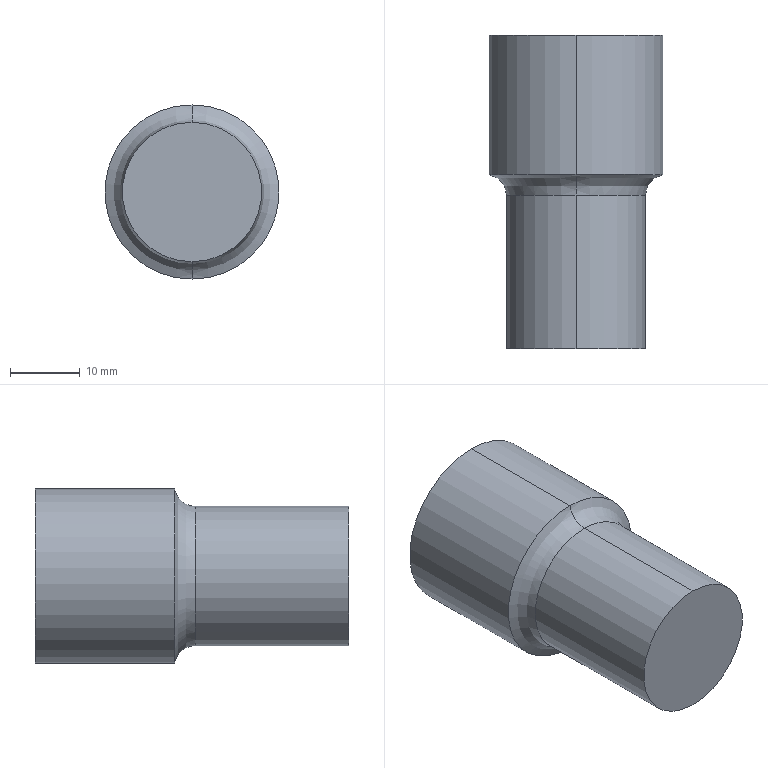Part | SolidWorks | features Fillet 1, Revolution 1 | 1 solid | 8 faces | box 25 x 45 x 25 mm | volume 17793 mm3 | cylinder 4 | torus 2 | plane 2 | commonest cylinder face diameters 20 x2 25 x2
STEP:
#1=CARTESIAN_POINT('',(0.,-6.354,-12.5));
#2=VERTEX_POINT('',#1);
#3=CARTESIAN_POINT('',(0.,-6.354,12.5));
#4=VERTEX_POINT('',#3);
#5=CARTESIAN_POINT('',(0.,-6.354,0.));
#6=DIRECTION('',(0.,1.,0.));
#7=DIRECTION('',(0.,0.,1.));
#8=AXIS2_PLACEMENT_3D('',#5,#6,#7);
#9=CIRCLE('',#8,12.5);
#10=EDGE_CURVE('',#2,#4,#9,.T.);
#11=ORIENTED_EDGE('',*,*,#10,.F.);
#12=CARTESIAN_POINT('',(0.,-9.312,-10.));
#13=VERTEX_POINT('',#12);
#14=CARTESIAN_POINT('',(0.,-9.312,-13.));
#15=DIRECTION('',(1.,0.,0.));
#16=DIRECTION('',(0.,0.,-1.));
#17=AXIS2_PLACEMENT_3D('',#14,#15,#16);
#18=CIRCLE('',#17,3.);
#19=EDGE_CURVE('',#2,#13,#18,.T.);
#20=ORIENTED_EDGE('',*,*,#19,.T.);
#21=CARTESIAN_POINT('',(0.,-9.312,10.));
#22=VERTEX_POINT('',#21);
#23=CARTESIAN_POINT('',(0.,-9.312,0.));
#24=DIRECTION('',(0.,-1.,0.));
#25=DIRECTION('',(0.,0.,1.));
#26=AXIS2_PLACEMENT_3D('',#23,#24,#25);
#27=CIRCLE('',#26,10.);
#28=EDGE_CURVE('',#22,#13,#27,.T.);
#29=ORIENTED_EDGE('',*,*,#28,.F.);
#30=CARTESIAN_POINT('',(0.,-9.312,13.));
#31=DIRECTION('',(-1.,0.,0.));
#32=DIRECTION('',(0.,0.,1.));
#33=AXIS2_PLACEMENT_3D('',#30,#31,#32);
#34=CIRCLE('',#33,3.);
#35=EDGE_CURVE('',#4,#22,#34,.T.);
#36=ORIENTED_EDGE('',*,*,#35,.F.);
#37=EDGE_LOOP('',(#11,#20,#29,#36));
#38=FACE_OUTER_BOUND('',#37,.T.);
#39=CARTESIAN_POINT('',(0.,-9.312,0.));
#40=DIRECTION('',(0.,1.,0.));
#41=DIRECTION('',(0.,0.,1.));
#42=AXIS2_PLACEMENT_3D('',#39,#40,#41);
#43=TOROIDAL_SURFACE('',#42,13.,3.);
#44=ADVANCED_FACE('',(#38),#43,.F.);
#45=CARTESIAN_POINT('',(0.,-31.354,10.));
#46=VERTEX_POINT('',#45);
#47=CARTESIAN_POINT('',(0.,-31.354,-10.));
#48=VERTEX_POINT('',#47);
#49=CARTESIAN_POINT('',(0.,-31.354,0.));
#50=DIRECTION('',(0.,1.,0.));
#51=DIRECTION('',(0.,0.,1.));
#52=AXIS2_PLACEMENT_3D('',#49,#50,#51);
#53=CIRCLE('',#52,10.);
#54=EDGE_CURVE('',#46,#48,#53,.T.);
#55=ORIENTED_EDGE('',*,*,#54,.T.);
#56=CARTESIAN_POINT('',(0.,17.049,-10.));
#57=DIRECTION('',(0.,1.,0.));
#58=VECTOR('',#57,1000.);
#59=LINE('',#56,#58);
#60=EDGE_CURVE('',#48,#13,#59,.T.);
#61=ORIENTED_EDGE('',*,*,#60,.T.);
#62=CARTESIAN_POINT('',(0.,-9.312,0.));
#63=DIRECTION('',(0.,-1.,0.));
#64=DIRECTION('',(0.,0.,1.));
#65=AXIS2_PLACEMENT_3D('',#62,#63,#64);
#66=CIRCLE('',#65,10.);
#67=EDGE_CURVE('',#13,#22,#66,.T.);
#68=ORIENTED_EDGE('',*,*,#67,.T.);
#69=CARTESIAN_POINT('',(0.,17.049,10.));
#70=DIRECTION('',(0.,1.,0.));
#71=VECTOR('',#70,1000.);
#72=LINE('',#69,#71);
#73=EDGE_CURVE('',#46,#22,#72,.T.);
#74=ORIENTED_EDGE('',*,*,#73,.F.);
#75=EDGE_LOOP('',(#55,#61,#68,#74));
#76=FACE_OUTER_BOUND('',#75,.T.);
#77=CARTESIAN_POINT('',(0.,17.049,0.));
#78=DIRECTION('',(0.,1.,0.));
#79=DIRECTION('',(0.,0.,1.));
#80=AXIS2_PLACEMENT_3D('',#77,#78,#79);
#81=CYLINDRICAL_SURFACE('',#80,10.);
#82=ADVANCED_FACE('',(#76),#81,.T.);
#83=CARTESIAN_POINT('',(0.,-6.354,0.));
#84=DIRECTION('',(0.,1.,0.));
#85=DIRECTION('',(0.,0.,1.));
#86=AXIS2_PLACEMENT_3D('',#83,#84,#85);
#87=CIRCLE('',#86,12.5);
#88=EDGE_CURVE('',#4,#2,#87,.T.);
#89=ORIENTED_EDGE('',*,*,#88,.T.);
#90=CARTESIAN_POINT('',(0.,13.646,-12.5));
#91=VERTEX_POINT('',#90);
#92=CARTESIAN_POINT('',(0.,17.049,-12.5));
#93=DIRECTION('',(0.,1.,0.));
#94=VECTOR('',#93,1000.);
#95=LINE('',#92,#94);
#96=EDGE_CURVE('',#2,#91,#95,.T.);
#97=ORIENTED_EDGE('',*,*,#96,.T.);
#98=CARTESIAN_POINT('',(0.,13.646,12.5));
#99=VERTEX_POINT('',#98);
#100=CARTESIAN_POINT('',(0.,13.646,0.));
#101=DIRECTION('',(0.,1.,0.));
#102=DIRECTION('',(0.,0.,1.));
#103=AXIS2_PLACEMENT_3D('',#100,#101,#102);
#104=CIRCLE('',#103,12.5);
#105=EDGE_CURVE('',#99,#91,#104,.T.);
#106=ORIENTED_EDGE('',*,*,#105,.F.);
#107=CARTESIAN_POINT('',(0.,17.049,12.5));
#108=DIRECTION('',(0.,1.,0.));
#109=VECTOR('',#108,1000.);
#110=LINE('',#107,#109);
#111=EDGE_CURVE('',#4,#99,#110,.T.);
#112=ORIENTED_EDGE('',*,*,#111,.F.);
#113=EDGE_LOOP('',(#89,#97,#106,#112));
#114=FACE_OUTER_BOUND('',#113,.T.);
#115=CARTESIAN_POINT('',(0.,17.049,0.));
#116=DIRECTION('',(0.,1.,0.));
#117=DIRECTION('',(0.,0.,1.));
#118=AXIS2_PLACEMENT_3D('',#115,#116,#117);
#119=CYLINDRICAL_SURFACE('',#118,12.5);
#120=ADVANCED_FACE('',(#114),#119,.T.);
#121=ORIENTED_EDGE('',*,*,#105,.T.);
#122=CARTESIAN_POINT('',(0.,13.646,0.));
#123=DIRECTION('',(0.,1.,0.));
#124=DIRECTION('',(0.,0.,1.));
#125=AXIS2_PLACEMENT_3D('',#122,#123,#124);
#126=CIRCLE('',#125,12.5);
#127=EDGE_CURVE('',#91,#99,#126,.T.);
#128=ORIENTED_EDGE('',*,*,#127,.T.);
#129=EDGE_LOOP('',(#121,#128));
#130=FACE_OUTER_BOUND('',#129,.T.);
#131=CARTESIAN_POINT('',(0.,13.646,0.));
#132=DIRECTION('',(0.,1.,0.));
#133=DIRECTION('',(0.,0.,1.));
#134=AXIS2_PLACEMENT_3D('',#131,#132,#133);
#135=PLANE('',#134);
#136=ADVANCED_FACE('',(#130),#135,.T.);
#137=ORIENTED_EDGE('',*,*,#96,.F.);
#138=ORIENTED_EDGE('',*,*,#10,.T.);
#139=ORIENTED_EDGE('',*,*,#111,.T.);
#140=ORIENTED_EDGE('',*,*,#127,.F.);
#141=EDGE_LOOP('',(#137,#138,#139,#140));
#142=FACE_OUTER_BOUND('',#141,.T.);
#143=CARTESIAN_POINT('',(0.,17.049,0.));
#144=DIRECTION('',(0.,1.,0.));
#145=DIRECTION('',(0.,0.,1.));
#146=AXIS2_PLACEMENT_3D('',#143,#144,#145);
#147=CYLINDRICAL_SURFACE('',#146,12.5);
#148=ADVANCED_FACE('',(#142),#147,.T.);
#149=ORIENTED_EDGE('',*,*,#54,.F.);
#150=CARTESIAN_POINT('',(0.,-31.354,0.));
#151=DIRECTION('',(0.,1.,0.));
#152=DIRECTION('',(0.,0.,1.));
#153=AXIS2_PLACEMENT_3D('',#150,#151,#152);
#154=CIRCLE('',#153,10.);
#155=EDGE_CURVE('',#48,#46,#154,.T.);
#156=ORIENTED_EDGE('',*,*,#155,.F.);
#157=EDGE_LOOP('',(#149,#156));
#158=FACE_OUTER_BOUND('',#157,.T.);
#159=CARTESIAN_POINT('',(0.,-31.354,0.));
#160=DIRECTION('',(0.,1.,0.));
#161=DIRECTION('',(0.,0.,1.));
#162=AXIS2_PLACEMENT_3D('',#159,#160,#161);
#163=PLANE('',#162);
#164=ADVANCED_FACE('',(#158),#163,.F.);
#165=ORIENTED_EDGE('',*,*,#60,.F.);
#166=ORIENTED_EDGE('',*,*,#155,.T.);
#167=ORIENTED_EDGE('',*,*,#73,.T.);
#168=ORIENTED_EDGE('',*,*,#28,.T.);
#169=EDGE_LOOP('',(#165,#166,#167,#168));
#170=FACE_OUTER_BOUND('',#169,.T.);
#171=CARTESIAN_POINT('',(0.,17.049,0.));
#172=DIRECTION('',(0.,1.,0.));
#173=DIRECTION('',(0.,0.,1.));
#174=AXIS2_PLACEMENT_3D('',#171,#172,#173);
#175=CYLINDRICAL_SURFACE('',#174,10.);
#176=ADVANCED_FACE('',(#170),#175,.T.);
#177=ORIENTED_EDGE('',*,*,#19,.F.);
#178=ORIENTED_EDGE('',*,*,#88,.F.);
#179=ORIENTED_EDGE('',*,*,#35,.T.);
#180=ORIENTED_EDGE('',*,*,#67,.F.);
#181=EDGE_LOOP('',(#177,#178,#179,#180));
#182=FACE_OUTER_BOUND('',#181,.T.);
#183=CARTESIAN_POINT('',(0.,-9.312,0.));
#184=DIRECTION('',(0.,1.,0.));
#185=DIRECTION('',(0.,0.,1.));
#186=AXIS2_PLACEMENT_3D('',#183,#184,#185);
#187=TOROIDAL_SURFACE('',#186,13.,3.);
#188=ADVANCED_FACE('',(#182),#187,.F.);
#189=CLOSED_SHELL('',(#44,#82,#120,#136,#148,#164,#176,#188));
#190=MANIFOLD_SOLID_BREP('',#189);
#191=CARTESIAN_POINT('',(0.,0.,0.));
#192=DIRECTION('',(0.,0.,1.));
#193=DIRECTION('',(1.,0.,0.));
#194=AXIS2_PLACEMENT_3D('',#191,#192,#193);
#195=(LENGTH_UNIT()NAMED_UNIT(*)SI_UNIT(.MILLI.,.METRE.));
#196=UNCERTAINTY_MEASURE_WITH_UNIT(LENGTH_MEASURE(0.00001),#195,'','');
#197=(NAMED_UNIT(*)PLANE_ANGLE_UNIT()SI_UNIT($,.RADIAN.));
#198=(NAMED_UNIT(*)SI_UNIT($,.STERADIAN.)SOLID_ANGLE_UNIT());
#199=(GEOMETRIC_REPRESENTATION_CONTEXT(3)GLOBAL_UNCERTAINTY_ASSIGNED_CONTEXT((#196))GLOBAL_UNIT_ASSIGNED_CONTEXT((#195,#197,#198))REPRESENTATION_CONTEXT('',''));
#200=ADVANCED_BREP_SHAPE_REPRESENTATION('',(#190,#194),#199);